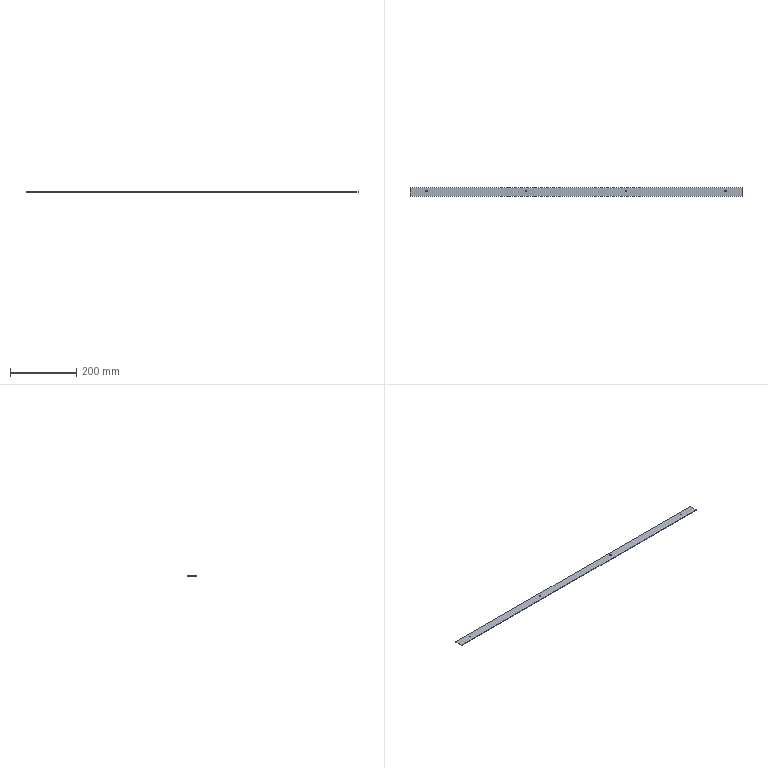Part | STEP file | 1 solid | 14 faces | box 1000 x 25 x 1.5 mm | volume 37405 mm3 | cylinder 8 | plane 6 | commonest cylinder face diameters 4.5 x8
STEP:
#1=CARTESIAN_POINT('',(0.,0.,0.));
#2=DIRECTION('',(0.,0.,1.));
#3=DIRECTION('',(1.,0.,0.));
#4=AXIS2_PLACEMENT_3D('',#1,#2,#3);
#5=CARTESIAN_POINT('',(782.25,-55.,1.5));
#6=VERTEX_POINT('',#5);
#7=CARTESIAN_POINT('',(777.75,-55.,1.5));
#8=VERTEX_POINT('',#7);
#9=CARTESIAN_POINT('',(780.,-55.,1.5));
#10=DIRECTION('',(0.,0.,1.));
#11=DIRECTION('',(1.,0.,0.));
#12=AXIS2_PLACEMENT_3D('',#9,#10,#11);
#13=CIRCLE('',#12,2.25);
#14=CARTESIAN_POINT('',(780.,-55.,1.5));
#15=DIRECTION('',(0.,0.,1.));
#16=DIRECTION('',(1.,0.,0.));
#17=AXIS2_PLACEMENT_3D('',#14,#15,#16);
#18=CYLINDRICAL_SURFACE('',#17,2.25);
#19=CARTESIAN_POINT('',(0.,0.));
#20=DIRECTION('',(1.,0.));
#21=VECTOR('',#20,1.);
#22=LINE('',#19,#21);
#23=(GEOMETRIC_REPRESENTATION_CONTEXT(2)PARAMETRIC_REPRESENTATION_CONTEXT()REPRESENTATION_CONTEXT('',''));
#24=DEFINITIONAL_REPRESENTATION('',(#22),#23);
#25=PCURVE('',#18,#24);
#26=CARTESIAN_POINT('',(0.,0.,1.5));
#27=DIRECTION('',(0.,0.,1.));
#28=DIRECTION('',(1.,0.,0.));
#29=AXIS2_PLACEMENT_3D('',#26,#27,#28);
#30=PLANE('',#29);
#31=CARTESIAN_POINT('',(780.,-55.));
#32=DIRECTION('',(1.,0.));
#33=AXIS2_PLACEMENT_2D('',#31,#32);
#34=CIRCLE('',#33,2.25);
#35=(GEOMETRIC_REPRESENTATION_CONTEXT(2)PARAMETRIC_REPRESENTATION_CONTEXT()REPRESENTATION_CONTEXT('',''));
#36=DEFINITIONAL_REPRESENTATION('',(#34),#35);
#37=PCURVE('',#30,#36);
#38=SURFACE_CURVE('',#13,(#25,#37),.PCURVE_S1.);
#39=EDGE_CURVE('',#6,#8,#38,.T.);
#40=ORIENTED_EDGE('',*,*,#39,.F.);
#41=CARTESIAN_POINT('',(782.25,-55.,0.));
#42=VERTEX_POINT('',#41);
#43=CARTESIAN_POINT('',(782.25,-55.,1.5));
#44=DIRECTION('',(0.,0.,1.));
#45=VECTOR('',#44,1.);
#46=LINE('',#43,#45);
#47=CARTESIAN_POINT('',(0.,0.));
#48=DIRECTION('',(0.,1.));
#49=VECTOR('',#48,1.);
#50=LINE('',#47,#49);
#51=(GEOMETRIC_REPRESENTATION_CONTEXT(2)PARAMETRIC_REPRESENTATION_CONTEXT()REPRESENTATION_CONTEXT('',''));
#52=DEFINITIONAL_REPRESENTATION('',(#50),#51);
#53=PCURVE('',#18,#52);
#54=CARTESIAN_POINT('',(780.,-55.,1.5));
#55=DIRECTION('',(0.,0.,1.));
#56=DIRECTION('',(1.,0.,0.));
#57=AXIS2_PLACEMENT_3D('',#54,#55,#56);
#58=CYLINDRICAL_SURFACE('',#57,2.25);
#59=CARTESIAN_POINT('',(6.283,0.));
#60=DIRECTION('',(0.,1.));
#61=VECTOR('',#60,1.);
#62=LINE('',#59,#61);
#63=(GEOMETRIC_REPRESENTATION_CONTEXT(2)PARAMETRIC_REPRESENTATION_CONTEXT()REPRESENTATION_CONTEXT('',''));
#64=DEFINITIONAL_REPRESENTATION('',(#62),#63);
#65=PCURVE('',#58,#64);
#66=SURFACE_CURVE('',#46,(#53,#65),.PCURVE_S1.);
#67=EDGE_CURVE('',#42,#6,#66,.T.);
#68=ORIENTED_EDGE('',*,*,#67,.F.);
#69=CARTESIAN_POINT('',(777.75,-55.,0.));
#70=VERTEX_POINT('',#69);
#71=CARTESIAN_POINT('',(780.,-55.,0.));
#72=DIRECTION('',(0.,0.,1.));
#73=DIRECTION('',(1.,0.,0.));
#74=AXIS2_PLACEMENT_3D('',#71,#72,#73);
#75=CIRCLE('',#74,2.25);
#76=CARTESIAN_POINT('',(0.,-1.5));
#77=DIRECTION('',(1.,0.));
#78=VECTOR('',#77,1.);
#79=LINE('',#76,#78);
#80=(GEOMETRIC_REPRESENTATION_CONTEXT(2)PARAMETRIC_REPRESENTATION_CONTEXT()REPRESENTATION_CONTEXT('',''));
#81=DEFINITIONAL_REPRESENTATION('',(#79),#80);
#82=PCURVE('',#18,#81);
#83=CARTESIAN_POINT('',(0.,0.,0.));
#84=DIRECTION('',(0.,0.,1.));
#85=DIRECTION('',(1.,0.,0.));
#86=AXIS2_PLACEMENT_3D('',#83,#84,#85);
#87=PLANE('',#86);
#88=CARTESIAN_POINT('',(780.,-55.));
#89=DIRECTION('',(1.,0.));
#90=AXIS2_PLACEMENT_2D('',#88,#89);
#91=CIRCLE('',#90,2.25);
#92=(GEOMETRIC_REPRESENTATION_CONTEXT(2)PARAMETRIC_REPRESENTATION_CONTEXT()REPRESENTATION_CONTEXT('',''));
#93=DEFINITIONAL_REPRESENTATION('',(#91),#92);
#94=PCURVE('',#87,#93);
#95=SURFACE_CURVE('',#75,(#82,#94),.PCURVE_S1.);
#96=EDGE_CURVE('',#42,#70,#95,.T.);
#97=ORIENTED_EDGE('',*,*,#96,.T.);
#98=CARTESIAN_POINT('',(777.75,-55.,1.5));
#99=DIRECTION('',(0.,0.,1.));
#100=VECTOR('',#99,1.);
#101=LINE('',#98,#100);
#102=CARTESIAN_POINT('',(3.142,0.));
#103=DIRECTION('',(0.,1.));
#104=VECTOR('',#103,1.);
#105=LINE('',#102,#104);
#106=(GEOMETRIC_REPRESENTATION_CONTEXT(2)PARAMETRIC_REPRESENTATION_CONTEXT()REPRESENTATION_CONTEXT('',''));
#107=DEFINITIONAL_REPRESENTATION('',(#105),#106);
#108=PCURVE('',#18,#107);
#109=CARTESIAN_POINT('',(3.142,0.));
#110=DIRECTION('',(0.,1.));
#111=VECTOR('',#110,1.);
#112=LINE('',#109,#111);
#113=(GEOMETRIC_REPRESENTATION_CONTEXT(2)PARAMETRIC_REPRESENTATION_CONTEXT()REPRESENTATION_CONTEXT('',''));
#114=DEFINITIONAL_REPRESENTATION('',(#112),#113);
#115=PCURVE('',#58,#114);
#116=SURFACE_CURVE('',#101,(#108,#115),.PCURVE_S1.);
#117=EDGE_CURVE('',#70,#8,#116,.T.);
#118=ORIENTED_EDGE('',*,*,#117,.T.);
#119=EDGE_LOOP('',(#40,#68,#97,#118));
#120=FACE_BOUND('',#119,.F.);
#121=ADVANCED_FACE('',(#120),#18,.F.);
#122=CARTESIAN_POINT('',(1082.25,-55.,1.5));
#123=VERTEX_POINT('',#122);
#124=CARTESIAN_POINT('',(1077.75,-55.,1.5));
#125=VERTEX_POINT('',#124);
#126=CARTESIAN_POINT('',(1080.,-55.,1.5));
#127=DIRECTION('',(0.,0.,1.));
#128=DIRECTION('',(1.,0.,0.));
#129=AXIS2_PLACEMENT_3D('',#126,#127,#128);
#130=CIRCLE('',#129,2.25);
#131=CARTESIAN_POINT('',(1080.,-55.,1.5));
#132=DIRECTION('',(0.,0.,1.));
#133=DIRECTION('',(1.,0.,0.));
#134=AXIS2_PLACEMENT_3D('',#131,#132,#133);
#135=CYLINDRICAL_SURFACE('',#134,2.25);
#136=CARTESIAN_POINT('',(0.,0.));
#137=DIRECTION('',(1.,0.));
#138=VECTOR('',#137,1.);
#139=LINE('',#136,#138);
#140=(GEOMETRIC_REPRESENTATION_CONTEXT(2)PARAMETRIC_REPRESENTATION_CONTEXT()REPRESENTATION_CONTEXT('',''));
#141=DEFINITIONAL_REPRESENTATION('',(#139),#140);
#142=PCURVE('',#135,#141);
#143=CARTESIAN_POINT('',(1080.,-55.));
#144=DIRECTION('',(1.,0.));
#145=AXIS2_PLACEMENT_2D('',#143,#144);
#146=CIRCLE('',#145,2.25);
#147=(GEOMETRIC_REPRESENTATION_CONTEXT(2)PARAMETRIC_REPRESENTATION_CONTEXT()REPRESENTATION_CONTEXT('',''));
#148=DEFINITIONAL_REPRESENTATION('',(#146),#147);
#149=PCURVE('',#30,#148);
#150=SURFACE_CURVE('',#130,(#142,#149),.PCURVE_S1.);
#151=EDGE_CURVE('',#123,#125,#150,.T.);
#152=ORIENTED_EDGE('',*,*,#151,.F.);
#153=CARTESIAN_POINT('',(1082.25,-55.,0.));
#154=VERTEX_POINT('',#153);
#155=CARTESIAN_POINT('',(1082.25,-55.,1.5));
#156=DIRECTION('',(0.,0.,1.));
#157=VECTOR('',#156,1.);
#158=LINE('',#155,#157);
#159=CARTESIAN_POINT('',(0.,0.));
#160=DIRECTION('',(0.,1.));
#161=VECTOR('',#160,1.);
#162=LINE('',#159,#161);
#163=(GEOMETRIC_REPRESENTATION_CONTEXT(2)PARAMETRIC_REPRESENTATION_CONTEXT()REPRESENTATION_CONTEXT('',''));
#164=DEFINITIONAL_REPRESENTATION('',(#162),#163);
#165=PCURVE('',#135,#164);
#166=CARTESIAN_POINT('',(1080.,-55.,1.5));
#167=DIRECTION('',(0.,0.,1.));
#168=DIRECTION('',(1.,0.,0.));
#169=AXIS2_PLACEMENT_3D('',#166,#167,#168);
#170=CYLINDRICAL_SURFACE('',#169,2.25);
#171=CARTESIAN_POINT('',(6.283,0.));
#172=DIRECTION('',(0.,1.));
#173=VECTOR('',#172,1.);
#174=LINE('',#171,#173);
#175=(GEOMETRIC_REPRESENTATION_CONTEXT(2)PARAMETRIC_REPRESENTATION_CONTEXT()REPRESENTATION_CONTEXT('',''));
#176=DEFINITIONAL_REPRESENTATION('',(#174),#175);
#177=PCURVE('',#170,#176);
#178=SURFACE_CURVE('',#158,(#165,#177),.PCURVE_S1.);
#179=EDGE_CURVE('',#154,#123,#178,.T.);
#180=ORIENTED_EDGE('',*,*,#179,.F.);
#181=CARTESIAN_POINT('',(1077.75,-55.,0.));
#182=VERTEX_POINT('',#181);
#183=CARTESIAN_POINT('',(1080.,-55.,0.));
#184=DIRECTION('',(0.,0.,1.));
#185=DIRECTION('',(1.,0.,0.));
#186=AXIS2_PLACEMENT_3D('',#183,#184,#185);
#187=CIRCLE('',#186,2.25);
#188=CARTESIAN_POINT('',(0.,-1.5));
#189=DIRECTION('',(1.,0.));
#190=VECTOR('',#189,1.);
#191=LINE('',#188,#190);
#192=(GEOMETRIC_REPRESENTATION_CONTEXT(2)PARAMETRIC_REPRESENTATION_CONTEXT()REPRESENTATION_CONTEXT('',''));
#193=DEFINITIONAL_REPRESENTATION('',(#191),#192);
#194=PCURVE('',#135,#193);
#195=CARTESIAN_POINT('',(1080.,-55.));
#196=DIRECTION('',(1.,0.));
#197=AXIS2_PLACEMENT_2D('',#195,#196);
#198=CIRCLE('',#197,2.25);
#199=(GEOMETRIC_REPRESENTATION_CONTEXT(2)PARAMETRIC_REPRESENTATION_CONTEXT()REPRESENTATION_CONTEXT('',''));
#200=DEFINITIONAL_REPRESENTATION('',(#198),#199);
#201=PCURVE('',#87,#200);
#202=SURFACE_CURVE('',#187,(#194,#201),.PCURVE_S1.);
#203=EDGE_CURVE('',#154,#182,#202,.T.);
#204=ORIENTED_EDGE('',*,*,#203,.T.);
#205=CARTESIAN_POINT('',(1077.75,-55.,1.5));
#206=DIRECTION('',(0.,0.,1.));
#207=VECTOR('',#206,1.);
#208=LINE('',#205,#207);
#209=CARTESIAN_POINT('',(3.142,0.));
#210=DIRECTION('',(0.,1.));
#211=VECTOR('',#210,1.);
#212=LINE('',#209,#211);
#213=(GEOMETRIC_REPRESENTATION_CONTEXT(2)PARAMETRIC_REPRESENTATION_CONTEXT()REPRESENTATION_CONTEXT('',''));
#214=DEFINITIONAL_REPRESENTATION('',(#212),#213);
#215=PCURVE('',#135,#214);
#216=CARTESIAN_POINT('',(3.142,0.));
#217=DIRECTION('',(0.,1.));
#218=VECTOR('',#217,1.);
#219=LINE('',#216,#218);
#220=(GEOMETRIC_REPRESENTATION_CONTEXT(2)PARAMETRIC_REPRESENTATION_CONTEXT()REPRESENTATION_CONTEXT('',''));
#221=DEFINITIONAL_REPRESENTATION('',(#219),#220);
#222=PCURVE('',#170,#221);
#223=SURFACE_CURVE('',#208,(#215,#222),.PCURVE_S1.);
#224=EDGE_CURVE('',#182,#125,#223,.T.);
#225=ORIENTED_EDGE('',*,*,#224,.T.);
#226=EDGE_LOOP('',(#152,#180,#204,#225));
#227=FACE_BOUND('',#226,.F.);
#228=ADVANCED_FACE('',(#227),#135,.F.);
#229=CARTESIAN_POINT('',(1382.25,-55.,1.5));
#230=VERTEX_POINT('',#229);
#231=CARTESIAN_POINT('',(1377.75,-55.,1.5));
#232=VERTEX_POINT('',#231);
#233=CARTESIAN_POINT('',(1380.,-55.,1.5));
#234=DIRECTION('',(0.,0.,1.));
#235=DIRECTION('',(1.,0.,0.));
#236=AXIS2_PLACEMENT_3D('',#233,#234,#235);
#237=CIRCLE('',#236,2.25);
#238=CARTESIAN_POINT('',(1380.,-55.,1.5));
#239=DIRECTION('',(0.,0.,1.));
#240=DIRECTION('',(1.,0.,0.));
#241=AXIS2_PLACEMENT_3D('',#238,#239,#240);
#242=CYLINDRICAL_SURFACE('',#241,2.25);
#243=CARTESIAN_POINT('',(0.,0.));
#244=DIRECTION('',(1.,0.));
#245=VECTOR('',#244,1.);
#246=LINE('',#243,#245);
#247=(GEOMETRIC_REPRESENTATION_CONTEXT(2)PARAMETRIC_REPRESENTATION_CONTEXT()REPRESENTATION_CONTEXT('',''));
#248=DEFINITIONAL_REPRESENTATION('',(#246),#247);
#249=PCURVE('',#242,#248);
#250=CARTESIAN_POINT('',(1380.,-55.));
#251=DIRECTION('',(1.,0.));
#252=AXIS2_PLACEMENT_2D('',#250,#251);
#253=CIRCLE('',#252,2.25);
#254=(GEOMETRIC_REPRESENTATION_CONTEXT(2)PARAMETRIC_REPRESENTATION_CONTEXT()REPRESENTATION_CONTEXT('',''));
#255=DEFINITIONAL_REPRESENTATION('',(#253),#254);
#256=PCURVE('',#30,#255);
#257=SURFACE_CURVE('',#237,(#249,#256),.PCURVE_S1.);
#258=EDGE_CURVE('',#230,#232,#257,.T.);
#259=ORIENTED_EDGE('',*,*,#258,.F.);
#260=CARTESIAN_POINT('',(1382.25,-55.,0.));
#261=VERTEX_POINT('',#260);
#262=CARTESIAN_POINT('',(1382.25,-55.,1.5));
#263=DIRECTION('',(0.,0.,1.));
#264=VECTOR('',#263,1.);
#265=LINE('',#262,#264);
#266=CARTESIAN_POINT('',(0.,0.));
#267=DIRECTION('',(0.,1.));
#268=VECTOR('',#267,1.);
#269=LINE('',#266,#268);
#270=(GEOMETRIC_REPRESENTATION_CONTEXT(2)PARAMETRIC_REPRESENTATION_CONTEXT()REPRESENTATION_CONTEXT('',''));
#271=DEFINITIONAL_REPRESENTATION('',(#269),#270);
#272=PCURVE('',#242,#271);
#273=CARTESIAN_POINT('',(1380.,-55.,1.5));
#274=DIRECTION('',(0.,0.,1.));
#275=DIRECTION('',(1.,0.,0.));
#276=AXIS2_PLACEMENT_3D('',#273,#274,#275);
#277=CYLINDRICAL_SURFACE('',#276,2.25);
#278=CARTESIAN_POINT('',(6.283,0.));
#279=DIRECTION('',(0.,1.));
#280=VECTOR('',#279,1.);
#281=LINE('',#278,#280);
#282=(GEOMETRIC_REPRESENTATION_CONTEXT(2)PARAMETRIC_REPRESENTATION_CONTEXT()REPRESENTATION_CONTEXT('',''));
#283=DEFINITIONAL_REPRESENTATION('',(#281),#282);
#284=PCURVE('',#277,#283);
#285=SURFACE_CURVE('',#265,(#272,#284),.PCURVE_S1.);
#286=EDGE_CURVE('',#261,#230,#285,.T.);
#287=ORIENTED_EDGE('',*,*,#286,.F.);
#288=CARTESIAN_POINT('',(1377.75,-55.,0.));
#289=VERTEX_POINT('',#288);
#290=CARTESIAN_POINT('',(1380.,-55.,0.));
#291=DIRECTION('',(0.,0.,1.));
#292=DIRECTION('',(1.,0.,0.));
#293=AXIS2_PLACEMENT_3D('',#290,#291,#292);
#294=CIRCLE('',#293,2.25);
#295=CARTESIAN_POINT('',(0.,-1.5));
#296=DIRECTION('',(1.,0.));
#297=VECTOR('',#296,1.);
#298=LINE('',#295,#297);
#299=(GEOMETRIC_REPRESENTATION_CONTEXT(2)PARAMETRIC_REPRESENTATION_CONTEXT()REPRESENTATION_CONTEXT('',''));
#300=DEFINITIONAL_REPRESENTATION('',(#298),#299);
#301=PCURVE('',#242,#300);
#302=CARTESIAN_POINT('',(1380.,-55.));
#303=DIRECTION('',(1.,0.));
#304=AXIS2_PLACEMENT_2D('',#302,#303);
#305=CIRCLE('',#304,2.25);
#306=(GEOMETRIC_REPRESENTATION_CONTEXT(2)PARAMETRIC_REPRESENTATION_CONTEXT()REPRESENTATION_CONTEXT('',''));
#307=DEFINITIONAL_REPRESENTATION('',(#305),#306);
#308=PCURVE('',#87,#307);
#309=SURFACE_CURVE('',#294,(#301,#308),.PCURVE_S1.);
#310=EDGE_CURVE('',#261,#289,#309,.T.);
#311=ORIENTED_EDGE('',*,*,#310,.T.);
#312=CARTESIAN_POINT('',(1377.75,-55.,1.5));
#313=DIRECTION('',(0.,0.,1.));
#314=VECTOR('',#313,1.);
#315=LINE('',#312,#314);
#316=CARTESIAN_POINT('',(3.142,0.));
#317=DIRECTION('',(0.,1.));
#318=VECTOR('',#317,1.);
#319=LINE('',#316,#318);
#320=(GEOMETRIC_REPRESENTATION_CONTEXT(2)PARAMETRIC_REPRESENTATION_CONTEXT()REPRESENTATION_CONTEXT('',''));
#321=DEFINITIONAL_REPRESENTATION('',(#319),#320);
#322=PCURVE('',#242,#321);
#323=CARTESIAN_POINT('',(3.142,0.));
#324=DIRECTION('',(0.,1.));
#325=VECTOR('',#324,1.);
#326=LINE('',#323,#325);
#327=(GEOMETRIC_REPRESENTATION_CONTEXT(2)PARAMETRIC_REPRESENTATION_CONTEXT()REPRESENTATION_CONTEXT('',''));
#328=DEFINITIONAL_REPRESENTATION('',(#326),#327);
#329=PCURVE('',#277,#328);
#330=SURFACE_CURVE('',#315,(#322,#329),.PCURVE_S1.);
#331=EDGE_CURVE('',#289,#232,#330,.T.);
#332=ORIENTED_EDGE('',*,*,#331,.T.);
#333=EDGE_LOOP('',(#259,#287,#311,#332));
#334=FACE_BOUND('',#333,.F.);
#335=ADVANCED_FACE('',(#334),#242,.F.);
#336=CARTESIAN_POINT('',(1682.25,-55.,1.5));
#337=VERTEX_POINT('',#336);
#338=CARTESIAN_POINT('',(1677.75,-55.,1.5));
#339=VERTEX_POINT('',#338);
#340=CARTESIAN_POINT('',(1680.,-55.,1.5));
#341=DIRECTION('',(0.,0.,1.));
#342=DIRECTION('',(1.,0.,0.));
#343=AXIS2_PLACEMENT_3D('',#340,#341,#342);
#344=CIRCLE('',#343,2.25);
#345=CARTESIAN_POINT('',(1680.,-55.,1.5));
#346=DIRECTION('',(0.,0.,1.));
#347=DIRECTION('',(1.,0.,0.));
#348=AXIS2_PLACEMENT_3D('',#345,#346,#347);
#349=CYLINDRICAL_SURFACE('',#348,2.25);
#350=CARTESIAN_POINT('',(0.,0.));
#351=DIRECTION('',(1.,0.));
#352=VECTOR('',#351,1.);
#353=LINE('',#350,#352);
#354=(GEOMETRIC_REPRESENTATION_CONTEXT(2)PARAMETRIC_REPRESENTATION_CONTEXT()REPRESENTATION_CONTEXT('',''));
#355=DEFINITIONAL_REPRESENTATION('',(#353),#354);
#356=PCURVE('',#349,#355);
#357=CARTESIAN_POINT('',(1680.,-55.));
#358=DIRECTION('',(1.,0.));
#359=AXIS2_PLACEMENT_2D('',#357,#358);
#360=CIRCLE('',#359,2.25);
#361=(GEOMETRIC_REPRESENTATION_CONTEXT(2)PARAMETRIC_REPRESENTATION_CONTEXT()REPRESENTATION_CONTEXT('',''));
#362=DEFINITIONAL_REPRESENTATION('',(#360),#361);
#363=PCURVE('',#30,#362);
#364=SURFACE_CURVE('',#344,(#356,#363),.PCURVE_S1.);
#365=EDGE_CURVE('',#337,#339,#364,.T.);
#366=ORIENTED_EDGE('',*,*,#365,.F.);
#367=CARTESIAN_POINT('',(1682.25,-55.,0.));
#368=VERTEX_POINT('',#367);
#369=CARTESIAN_POINT('',(1682.25,-55.,1.5));
#370=DIRECTION('',(0.,0.,1.));
#371=VECTOR('',#370,1.);
#372=LINE('',#369,#371);
#373=CARTESIAN_POINT('',(0.,0.));
#374=DIRECTION('',(0.,1.));
#375=VECTOR('',#374,1.);
#376=LINE('',#373,#375);
#377=(GEOMETRIC_REPRESENTATION_CONTEXT(2)PARAMETRIC_REPRESENTATION_CONTEXT()REPRESENTATION_CONTEXT('',''));
#378=DEFINITIONAL_REPRESENTATION('',(#376),#377);
#379=PCURVE('',#349,#378);
#380=CARTESIAN_POINT('',(1680.,-55.,1.5));
#381=DIRECTION('',(0.,0.,1.));
#382=DIRECTION('',(1.,0.,0.));
#383=AXIS2_PLACEMENT_3D('',#380,#381,#382);
#384=CYLINDRICAL_SURFACE('',#383,2.25);
#385=CARTESIAN_POINT('',(6.283,0.));
#386=DIRECTION('',(0.,1.));
#387=VECTOR('',#386,1.);
#388=LINE('',#385,#387);
#389=(GEOMETRIC_REPRESENTATION_CONTEXT(2)PARAMETRIC_REPRESENTATION_CONTEXT()REPRESENTATION_CONTEXT('',''));
#390=DEFINITIONAL_REPRESENTATION('',(#388),#389);
#391=PCURVE('',#384,#390);
#392=SURFACE_CURVE('',#372,(#379,#391),.PCURVE_S1.);
#393=EDGE_CURVE('',#368,#337,#392,.T.);
#394=ORIENTED_EDGE('',*,*,#393,.F.);
#395=CARTESIAN_POINT('',(1677.75,-55.,0.));
#396=VERTEX_POINT('',#395);
#397=CARTESIAN_POINT('',(1680.,-55.,0.));
#398=DIRECTION('',(0.,0.,1.));
#399=DIRECTION('',(1.,0.,0.));
#400=AXIS2_PLACEMENT_3D('',#397,#398,#399);
#401=CIRCLE('',#400,2.25);
#402=CARTESIAN_POINT('',(0.,-1.5));
#403=DIRECTION('',(1.,0.));
#404=VECTOR('',#403,1.);
#405=LINE('',#402,#404);
#406=(GEOMETRIC_REPRESENTATION_CONTEXT(2)PARAMETRIC_REPRESENTATION_CONTEXT()REPRESENTATION_CONTEXT('',''));
#407=DEFINITIONAL_REPRESENTATION('',(#405),#406);
#408=PCURVE('',#349,#407);
#409=CARTESIAN_POINT('',(1680.,-55.));
#410=DIRECTION('',(1.,0.));
#411=AXIS2_PLACEMENT_2D('',#409,#410);
#412=CIRCLE('',#411,2.25);
#413=(GEOMETRIC_REPRESENTATION_CONTEXT(2)PARAMETRIC_REPRESENTATION_CONTEXT()REPRESENTATION_CONTEXT('',''));
#414=DEFINITIONAL_REPRESENTATION('',(#412),#413);
#415=PCURVE('',#87,#414);
#416=SURFACE_CURVE('',#401,(#408,#415),.PCURVE_S1.);
#417=EDGE_CURVE('',#368,#396,#416,.T.);
#418=ORIENTED_EDGE('',*,*,#417,.T.);
#419=CARTESIAN_POINT('',(1677.75,-55.,1.5));
#420=DIRECTION('',(0.,0.,1.));
#421=VECTOR('',#420,1.);
#422=LINE('',#419,#421);
#423=CARTESIAN_POINT('',(3.142,0.));
#424=DIRECTION('',(0.,1.));
#425=VECTOR('',#424,1.);
#426=LINE('',#423,#425);
#427=(GEOMETRIC_REPRESENTATION_CONTEXT(2)PARAMETRIC_REPRESENTATION_CONTEXT()REPRESENTATION_CONTEXT('',''));
#428=DEFINITIONAL_REPRESENTATION('',(#426),#427);
#429=PCURVE('',#349,#428);
#430=CARTESIAN_POINT('',(3.142,0.));
#431=DIRECTION('',(0.,1.));
#432=VECTOR('',#431,1.);
#433=LINE('',#430,#432);
#434=(GEOMETRIC_REPRESENTATION_CONTEXT(2)PARAMETRIC_REPRESENTATION_CONTEXT()REPRESENTATION_CONTEXT('',''));
#435=DEFINITIONAL_REPRESENTATION('',(#433),#434);
#436=PCURVE('',#384,#435);
#437=SURFACE_CURVE('',#422,(#429,#436),.PCURVE_S1.);
#438=EDGE_CURVE('',#396,#339,#437,.T.);
#439=ORIENTED_EDGE('',*,*,#438,.T.);
#440=EDGE_LOOP('',(#366,#394,#418,#439));
#441=FACE_BOUND('',#440,.F.);
#442=ADVANCED_FACE('',(#441),#349,.F.);
#443=ORIENTED_EDGE('',*,*,#417,.T.);
#444=CARTESIAN_POINT('',(1680.,-55.,0.));
#445=DIRECTION('',(0.,0.,1.));
#446=DIRECTION('',(1.,0.,0.));
#447=AXIS2_PLACEMENT_3D('',#444,#445,#446);
#448=CIRCLE('',#447,2.25);
#449=CARTESIAN_POINT('',(1680.,-55.));
#450=DIRECTION('',(1.,0.));
#451=AXIS2_PLACEMENT_2D('',#449,#450);
#452=CIRCLE('',#451,2.25);
#453=(GEOMETRIC_REPRESENTATION_CONTEXT(2)PARAMETRIC_REPRESENTATION_CONTEXT()REPRESENTATION_CONTEXT('',''));
#454=DEFINITIONAL_REPRESENTATION('',(#452),#453);
#455=PCURVE('',#87,#454);
#456=CARTESIAN_POINT('',(0.,-1.5));
#457=DIRECTION('',(1.,0.));
#458=VECTOR('',#457,1.);
#459=LINE('',#456,#458);
#460=(GEOMETRIC_REPRESENTATION_CONTEXT(2)PARAMETRIC_REPRESENTATION_CONTEXT()REPRESENTATION_CONTEXT('',''));
#461=DEFINITIONAL_REPRESENTATION('',(#459),#460);
#462=PCURVE('',#384,#461);
#463=SURFACE_CURVE('',#448,(#455,#462),.PCURVE_S1.);
#464=EDGE_CURVE('',#396,#368,#463,.T.);
#465=ORIENTED_EDGE('',*,*,#464,.T.);
#466=EDGE_LOOP('',(#443,#465));
#467=FACE_BOUND('',#466,.T.);
#468=ORIENTED_EDGE('',*,*,#310,.T.);
#469=CARTESIAN_POINT('',(1380.,-55.,0.));
#470=DIRECTION('',(0.,0.,1.));
#471=DIRECTION('',(1.,0.,0.));
#472=AXIS2_PLACEMENT_3D('',#469,#470,#471);
#473=CIRCLE('',#472,2.25);
#474=CARTESIAN_POINT('',(1380.,-55.));
#475=DIRECTION('',(1.,0.));
#476=AXIS2_PLACEMENT_2D('',#474,#475);
#477=CIRCLE('',#476,2.25);
#478=(GEOMETRIC_REPRESENTATION_CONTEXT(2)PARAMETRIC_REPRESENTATION_CONTEXT()REPRESENTATION_CONTEXT('',''));
#479=DEFINITIONAL_REPRESENTATION('',(#477),#478);
#480=PCURVE('',#87,#479);
#481=CARTESIAN_POINT('',(0.,-1.5));
#482=DIRECTION('',(1.,0.));
#483=VECTOR('',#482,1.);
#484=LINE('',#481,#483);
#485=(GEOMETRIC_REPRESENTATION_CONTEXT(2)PARAMETRIC_REPRESENTATION_CONTEXT()REPRESENTATION_CONTEXT('',''));
#486=DEFINITIONAL_REPRESENTATION('',(#484),#485);
#487=PCURVE('',#277,#486);
#488=SURFACE_CURVE('',#473,(#480,#487),.PCURVE_S1.);
#489=EDGE_CURVE('',#289,#261,#488,.T.);
#490=ORIENTED_EDGE('',*,*,#489,.T.);
#491=EDGE_LOOP('',(#468,#490));
#492=FACE_BOUND('',#491,.T.);
#493=ORIENTED_EDGE('',*,*,#203,.T.);
#494=CARTESIAN_POINT('',(1080.,-55.,0.));
#495=DIRECTION('',(0.,0.,1.));
#496=DIRECTION('',(1.,0.,0.));
#497=AXIS2_PLACEMENT_3D('',#494,#495,#496);
#498=CIRCLE('',#497,2.25);
#499=CARTESIAN_POINT('',(1080.,-55.));
#500=DIRECTION('',(1.,0.));
#501=AXIS2_PLACEMENT_2D('',#499,#500);
#502=CIRCLE('',#501,2.25);
#503=(GEOMETRIC_REPRESENTATION_CONTEXT(2)PARAMETRIC_REPRESENTATION_CONTEXT()REPRESENTATION_CONTEXT('',''));
#504=DEFINITIONAL_REPRESENTATION('',(#502),#503);
#505=PCURVE('',#87,#504);
#506=CARTESIAN_POINT('',(0.,-1.5));
#507=DIRECTION('',(1.,0.));
#508=VECTOR('',#507,1.);
#509=LINE('',#506,#508);
#510=(GEOMETRIC_REPRESENTATION_CONTEXT(2)PARAMETRIC_REPRESENTATION_CONTEXT()REPRESENTATION_CONTEXT('',''));
#511=DEFINITIONAL_REPRESENTATION('',(#509),#510);
#512=PCURVE('',#170,#511);
#513=SURFACE_CURVE('',#498,(#505,#512),.PCURVE_S1.);
#514=EDGE_CURVE('',#182,#154,#513,.T.);
#515=ORIENTED_EDGE('',*,*,#514,.T.);
#516=EDGE_LOOP('',(#493,#515));
#517=FACE_BOUND('',#516,.T.);
#518=ORIENTED_EDGE('',*,*,#96,.T.);
#519=CARTESIAN_POINT('',(780.,-55.,0.));
#520=DIRECTION('',(0.,0.,1.));
#521=DIRECTION('',(1.,0.,0.));
#522=AXIS2_PLACEMENT_3D('',#519,#520,#521);
#523=CIRCLE('',#522,2.25);
#524=CARTESIAN_POINT('',(780.,-55.));
#525=DIRECTION('',(1.,0.));
#526=AXIS2_PLACEMENT_2D('',#524,#525);
#527=CIRCLE('',#526,2.25);
#528=(GEOMETRIC_REPRESENTATION_CONTEXT(2)PARAMETRIC_REPRESENTATION_CONTEXT()REPRESENTATION_CONTEXT('',''));
#529=DEFINITIONAL_REPRESENTATION('',(#527),#528);
#530=PCURVE('',#87,#529);
#531=CARTESIAN_POINT('',(0.,-1.5));
#532=DIRECTION('',(1.,0.));
#533=VECTOR('',#532,1.);
#534=LINE('',#531,#533);
#535=(GEOMETRIC_REPRESENTATION_CONTEXT(2)PARAMETRIC_REPRESENTATION_CONTEXT()REPRESENTATION_CONTEXT('',''));
#536=DEFINITIONAL_REPRESENTATION('',(#534),#535);
#537=PCURVE('',#58,#536);
#538=SURFACE_CURVE('',#523,(#530,#537),.PCURVE_S1.);
#539=EDGE_CURVE('',#70,#42,#538,.T.);
#540=ORIENTED_EDGE('',*,*,#539,.T.);
#541=EDGE_LOOP('',(#518,#540));
#542=FACE_BOUND('',#541,.T.);
#543=CARTESIAN_POINT('',(1730.,-45.,0.));
#544=VERTEX_POINT('',#543);
#545=CARTESIAN_POINT('',(730.,-45.,0.));
#546=VERTEX_POINT('',#545);
#547=CARTESIAN_POINT('',(1500.,-45.,0.));
#548=DIRECTION('',(-1.,0.,0.));
#549=VECTOR('',#548,1.);
#550=LINE('',#547,#549);
#551=CARTESIAN_POINT('',(1500.,-45.));
#552=DIRECTION('',(-1.,0.));
#553=VECTOR('',#552,1.);
#554=LINE('',#551,#553);
#555=(GEOMETRIC_REPRESENTATION_CONTEXT(2)PARAMETRIC_REPRESENTATION_CONTEXT()REPRESENTATION_CONTEXT('',''));
#556=DEFINITIONAL_REPRESENTATION('',(#554),#555);
#557=PCURVE('',#87,#556);
#558=CARTESIAN_POINT('',(1500.,-45.,1.5));
#559=DIRECTION('',(0.,-1.,0.));
#560=DIRECTION('',(0.,0.,-1.));
#561=AXIS2_PLACEMENT_3D('',#558,#559,#560);
#562=PLANE('',#561);
#563=CARTESIAN_POINT('',(1.5,0.));
#564=DIRECTION('',(0.,-1.));
#565=VECTOR('',#564,1.);
#566=LINE('',#563,#565);
#567=(GEOMETRIC_REPRESENTATION_CONTEXT(2)PARAMETRIC_REPRESENTATION_CONTEXT()REPRESENTATION_CONTEXT('',''));
#568=DEFINITIONAL_REPRESENTATION('',(#566),#567);
#569=PCURVE('',#562,#568);
#570=SURFACE_CURVE('',#550,(#557,#569),.PCURVE_S1.);
#571=EDGE_CURVE('',#544,#546,#570,.T.);
#572=ORIENTED_EDGE('',*,*,#571,.F.);
#573=CARTESIAN_POINT('',(1730.,-70.,0.));
#574=VERTEX_POINT('',#573);
#575=CARTESIAN_POINT('',(1730.,-70.,0.));
#576=DIRECTION('',(0.,1.,0.));
#577=VECTOR('',#576,1.);
#578=LINE('',#575,#577);
#579=CARTESIAN_POINT('',(1730.,-70.));
#580=DIRECTION('',(0.,1.));
#581=VECTOR('',#580,1.);
#582=LINE('',#579,#581);
#583=(GEOMETRIC_REPRESENTATION_CONTEXT(2)PARAMETRIC_REPRESENTATION_CONTEXT()REPRESENTATION_CONTEXT('',''));
#584=DEFINITIONAL_REPRESENTATION('',(#582),#583);
#585=PCURVE('',#87,#584);
#586=CARTESIAN_POINT('',(1730.,-70.,1.5));
#587=DIRECTION('',(-1.,0.,0.));
#588=DIRECTION('',(0.,0.,1.));
#589=AXIS2_PLACEMENT_3D('',#586,#587,#588);
#590=PLANE('',#589);
#591=CARTESIAN_POINT('',(-1.5,0.));
#592=DIRECTION('',(0.,1.));
#593=VECTOR('',#592,1.);
#594=LINE('',#591,#593);
#595=(GEOMETRIC_REPRESENTATION_CONTEXT(2)PARAMETRIC_REPRESENTATION_CONTEXT()REPRESENTATION_CONTEXT('',''));
#596=DEFINITIONAL_REPRESENTATION('',(#594),#595);
#597=PCURVE('',#590,#596);
#598=SURFACE_CURVE('',#578,(#585,#597),.PCURVE_S1.);
#599=EDGE_CURVE('',#574,#544,#598,.T.);
#600=ORIENTED_EDGE('',*,*,#599,.F.);
#601=CARTESIAN_POINT('',(730.,-70.,0.));
#602=VERTEX_POINT('',#601);
#603=CARTESIAN_POINT('',(600.,-70.,0.));
#604=DIRECTION('',(1.,0.,0.));
#605=VECTOR('',#604,1.);
#606=LINE('',#603,#605);
#607=CARTESIAN_POINT('',(600.,-70.));
#608=DIRECTION('',(1.,0.));
#609=VECTOR('',#608,1.);
#610=LINE('',#607,#609);
#611=(GEOMETRIC_REPRESENTATION_CONTEXT(2)PARAMETRIC_REPRESENTATION_CONTEXT()REPRESENTATION_CONTEXT('',''));
#612=DEFINITIONAL_REPRESENTATION('',(#610),#611);
#613=PCURVE('',#87,#612);
#614=CARTESIAN_POINT('',(600.,-70.,1.5));
#615=DIRECTION('',(0.,1.,0.));
#616=DIRECTION('',(1.,0.,0.));
#617=AXIS2_PLACEMENT_3D('',#614,#615,#616);
#618=PLANE('',#617);
#619=CARTESIAN_POINT('',(0.,1.5));
#620=DIRECTION('',(1.,0.));
#621=VECTOR('',#620,1.);
#622=LINE('',#619,#621);
#623=(GEOMETRIC_REPRESENTATION_CONTEXT(2)PARAMETRIC_REPRESENTATION_CONTEXT()REPRESENTATION_CONTEXT('',''));
#624=DEFINITIONAL_REPRESENTATION('',(#622),#623);
#625=PCURVE('',#618,#624);
#626=SURFACE_CURVE('',#606,(#613,#625),.PCURVE_S1.);
#627=EDGE_CURVE('',#602,#574,#626,.T.);
#628=ORIENTED_EDGE('',*,*,#627,.F.);
#629=CARTESIAN_POINT('',(730.,-45.,0.));
#630=DIRECTION('',(0.,-1.,0.));
#631=VECTOR('',#630,1.);
#632=LINE('',#629,#631);
#633=CARTESIAN_POINT('',(730.,-45.));
#634=DIRECTION('',(0.,-1.));
#635=VECTOR('',#634,1.);
#636=LINE('',#633,#635);
#637=(GEOMETRIC_REPRESENTATION_CONTEXT(2)PARAMETRIC_REPRESENTATION_CONTEXT()REPRESENTATION_CONTEXT('',''));
#638=DEFINITIONAL_REPRESENTATION('',(#636),#637);
#639=PCURVE('',#87,#638);
#640=CARTESIAN_POINT('',(730.,-45.,1.5));
#641=DIRECTION('',(1.,0.,0.));
#642=DIRECTION('',(0.,0.,1.));
#643=AXIS2_PLACEMENT_3D('',#640,#641,#642);
#644=PLANE('',#643);
#645=CARTESIAN_POINT('',(-1.5,0.));
#646=DIRECTION('',(0.,1.));
#647=VECTOR('',#646,1.);
#648=LINE('',#645,#647);
#649=(GEOMETRIC_REPRESENTATION_CONTEXT(2)PARAMETRIC_REPRESENTATION_CONTEXT()REPRESENTATION_CONTEXT('',''));
#650=DEFINITIONAL_REPRESENTATION('',(#648),#649);
#651=PCURVE('',#644,#650);
#652=SURFACE_CURVE('',#632,(#639,#651),.PCURVE_S1.);
#653=EDGE_CURVE('',#546,#602,#652,.T.);
#654=ORIENTED_EDGE('',*,*,#653,.F.);
#655=EDGE_LOOP('',(#572,#600,#628,#654));
#656=FACE_BOUND('',#655,.T.);
#657=ADVANCED_FACE('',(#467,#492,#517,#542,#656),#87,.F.);
#658=ORIENTED_EDGE('',*,*,#365,.F.);
#659=CARTESIAN_POINT('',(1680.,-55.,1.5));
#660=DIRECTION('',(0.,0.,1.));
#661=DIRECTION('',(1.,0.,0.));
#662=AXIS2_PLACEMENT_3D('',#659,#660,#661);
#663=CIRCLE('',#662,2.25);
#664=CARTESIAN_POINT('',(1680.,-55.));
#665=DIRECTION('',(1.,0.));
#666=AXIS2_PLACEMENT_2D('',#664,#665);
#667=CIRCLE('',#666,2.25);
#668=(GEOMETRIC_REPRESENTATION_CONTEXT(2)PARAMETRIC_REPRESENTATION_CONTEXT()REPRESENTATION_CONTEXT('',''));
#669=DEFINITIONAL_REPRESENTATION('',(#667),#668);
#670=PCURVE('',#30,#669);
#671=CARTESIAN_POINT('',(0.,0.));
#672=DIRECTION('',(1.,0.));
#673=VECTOR('',#672,1.);
#674=LINE('',#671,#673);
#675=(GEOMETRIC_REPRESENTATION_CONTEXT(2)PARAMETRIC_REPRESENTATION_CONTEXT()REPRESENTATION_CONTEXT('',''));
#676=DEFINITIONAL_REPRESENTATION('',(#674),#675);
#677=PCURVE('',#384,#676);
#678=SURFACE_CURVE('',#663,(#670,#677),.PCURVE_S1.);
#679=EDGE_CURVE('',#339,#337,#678,.T.);
#680=ORIENTED_EDGE('',*,*,#679,.F.);
#681=EDGE_LOOP('',(#658,#680));
#682=FACE_BOUND('',#681,.T.);
#683=ORIENTED_EDGE('',*,*,#258,.F.);
#684=CARTESIAN_POINT('',(1380.,-55.,1.5));
#685=DIRECTION('',(0.,0.,1.));
#686=DIRECTION('',(1.,0.,0.));
#687=AXIS2_PLACEMENT_3D('',#684,#685,#686);
#688=CIRCLE('',#687,2.25);
#689=CARTESIAN_POINT('',(1380.,-55.));
#690=DIRECTION('',(1.,0.));
#691=AXIS2_PLACEMENT_2D('',#689,#690);
#692=CIRCLE('',#691,2.25);
#693=(GEOMETRIC_REPRESENTATION_CONTEXT(2)PARAMETRIC_REPRESENTATION_CONTEXT()REPRESENTATION_CONTEXT('',''));
#694=DEFINITIONAL_REPRESENTATION('',(#692),#693);
#695=PCURVE('',#30,#694);
#696=CARTESIAN_POINT('',(0.,0.));
#697=DIRECTION('',(1.,0.));
#698=VECTOR('',#697,1.);
#699=LINE('',#696,#698);
#700=(GEOMETRIC_REPRESENTATION_CONTEXT(2)PARAMETRIC_REPRESENTATION_CONTEXT()REPRESENTATION_CONTEXT('',''));
#701=DEFINITIONAL_REPRESENTATION('',(#699),#700);
#702=PCURVE('',#277,#701);
#703=SURFACE_CURVE('',#688,(#695,#702),.PCURVE_S1.);
#704=EDGE_CURVE('',#232,#230,#703,.T.);
#705=ORIENTED_EDGE('',*,*,#704,.F.);
#706=EDGE_LOOP('',(#683,#705));
#707=FACE_BOUND('',#706,.T.);
#708=ORIENTED_EDGE('',*,*,#151,.F.);
#709=CARTESIAN_POINT('',(1080.,-55.,1.5));
#710=DIRECTION('',(0.,0.,1.));
#711=DIRECTION('',(1.,0.,0.));
#712=AXIS2_PLACEMENT_3D('',#709,#710,#711);
#713=CIRCLE('',#712,2.25);
#714=CARTESIAN_POINT('',(1080.,-55.));
#715=DIRECTION('',(1.,0.));
#716=AXIS2_PLACEMENT_2D('',#714,#715);
#717=CIRCLE('',#716,2.25);
#718=(GEOMETRIC_REPRESENTATION_CONTEXT(2)PARAMETRIC_REPRESENTATION_CONTEXT()REPRESENTATION_CONTEXT('',''));
#719=DEFINITIONAL_REPRESENTATION('',(#717),#718);
#720=PCURVE('',#30,#719);
#721=CARTESIAN_POINT('',(0.,0.));
#722=DIRECTION('',(1.,0.));
#723=VECTOR('',#722,1.);
#724=LINE('',#721,#723);
#725=(GEOMETRIC_REPRESENTATION_CONTEXT(2)PARAMETRIC_REPRESENTATION_CONTEXT()REPRESENTATION_CONTEXT('',''));
#726=DEFINITIONAL_REPRESENTATION('',(#724),#725);
#727=PCURVE('',#170,#726);
#728=SURFACE_CURVE('',#713,(#720,#727),.PCURVE_S1.);
#729=EDGE_CURVE('',#125,#123,#728,.T.);
#730=ORIENTED_EDGE('',*,*,#729,.F.);
#731=EDGE_LOOP('',(#708,#730));
#732=FACE_BOUND('',#731,.T.);
#733=ORIENTED_EDGE('',*,*,#39,.F.);
#734=CARTESIAN_POINT('',(780.,-55.,1.5));
#735=DIRECTION('',(0.,0.,1.));
#736=DIRECTION('',(1.,0.,0.));
#737=AXIS2_PLACEMENT_3D('',#734,#735,#736);
#738=CIRCLE('',#737,2.25);
#739=CARTESIAN_POINT('',(780.,-55.));
#740=DIRECTION('',(1.,0.));
#741=AXIS2_PLACEMENT_2D('',#739,#740);
#742=CIRCLE('',#741,2.25);
#743=(GEOMETRIC_REPRESENTATION_CONTEXT(2)PARAMETRIC_REPRESENTATION_CONTEXT()REPRESENTATION_CONTEXT('',''));
#744=DEFINITIONAL_REPRESENTATION('',(#742),#743);
#745=PCURVE('',#30,#744);
#746=CARTESIAN_POINT('',(0.,0.));
#747=DIRECTION('',(1.,0.));
#748=VECTOR('',#747,1.);
#749=LINE('',#746,#748);
#750=(GEOMETRIC_REPRESENTATION_CONTEXT(2)PARAMETRIC_REPRESENTATION_CONTEXT()REPRESENTATION_CONTEXT('',''));
#751=DEFINITIONAL_REPRESENTATION('',(#749),#750);
#752=PCURVE('',#58,#751);
#753=SURFACE_CURVE('',#738,(#745,#752),.PCURVE_S1.);
#754=EDGE_CURVE('',#8,#6,#753,.T.);
#755=ORIENTED_EDGE('',*,*,#754,.F.);
#756=EDGE_LOOP('',(#733,#755));
#757=FACE_BOUND('',#756,.T.);
#758=CARTESIAN_POINT('',(1730.,-45.,1.5));
#759=VERTEX_POINT('',#758);
#760=CARTESIAN_POINT('',(730.,-45.,1.5));
#761=VERTEX_POINT('',#760);
#762=CARTESIAN_POINT('',(1500.,-45.,1.5));
#763=DIRECTION('',(-1.,0.,0.));
#764=VECTOR('',#763,1.);
#765=LINE('',#762,#764);
#766=CARTESIAN_POINT('',(1500.,-45.));
#767=DIRECTION('',(-1.,0.));
#768=VECTOR('',#767,1.);
#769=LINE('',#766,#768);
#770=(GEOMETRIC_REPRESENTATION_CONTEXT(2)PARAMETRIC_REPRESENTATION_CONTEXT()REPRESENTATION_CONTEXT('',''));
#771=DEFINITIONAL_REPRESENTATION('',(#769),#770);
#772=PCURVE('',#30,#771);
#773=CARTESIAN_POINT('',(0.,0.));
#774=DIRECTION('',(0.,-1.));
#775=VECTOR('',#774,1.);
#776=LINE('',#773,#775);
#777=(GEOMETRIC_REPRESENTATION_CONTEXT(2)PARAMETRIC_REPRESENTATION_CONTEXT()REPRESENTATION_CONTEXT('',''));
#778=DEFINITIONAL_REPRESENTATION('',(#776),#777);
#779=PCURVE('',#562,#778);
#780=SURFACE_CURVE('',#765,(#772,#779),.PCURVE_S1.);
#781=EDGE_CURVE('',#759,#761,#780,.T.);
#782=ORIENTED_EDGE('',*,*,#781,.T.);
#783=CARTESIAN_POINT('',(730.,-70.,1.5));
#784=VERTEX_POINT('',#783);
#785=CARTESIAN_POINT('',(730.,-45.,1.5));
#786=DIRECTION('',(0.,-1.,0.));
#787=VECTOR('',#786,1.);
#788=LINE('',#785,#787);
#789=CARTESIAN_POINT('',(730.,-45.));
#790=DIRECTION('',(0.,-1.));
#791=VECTOR('',#790,1.);
#792=LINE('',#789,#791);
#793=(GEOMETRIC_REPRESENTATION_CONTEXT(2)PARAMETRIC_REPRESENTATION_CONTEXT()REPRESENTATION_CONTEXT('',''));
#794=DEFINITIONAL_REPRESENTATION('',(#792),#793);
#795=PCURVE('',#30,#794);
#796=CARTESIAN_POINT('',(0.,0.));
#797=DIRECTION('',(0.,1.));
#798=VECTOR('',#797,1.);
#799=LINE('',#796,#798);
#800=(GEOMETRIC_REPRESENTATION_CONTEXT(2)PARAMETRIC_REPRESENTATION_CONTEXT()REPRESENTATION_CONTEXT('',''));
#801=DEFINITIONAL_REPRESENTATION('',(#799),#800);
#802=PCURVE('',#644,#801);
#803=SURFACE_CURVE('',#788,(#795,#802),.PCURVE_S1.);
#804=EDGE_CURVE('',#761,#784,#803,.T.);
#805=ORIENTED_EDGE('',*,*,#804,.T.);
#806=CARTESIAN_POINT('',(1730.,-70.,1.5));
#807=VERTEX_POINT('',#806);
#808=CARTESIAN_POINT('',(600.,-70.,1.5));
#809=DIRECTION('',(1.,0.,0.));
#810=VECTOR('',#809,1.);
#811=LINE('',#808,#810);
#812=CARTESIAN_POINT('',(600.,-70.));
#813=DIRECTION('',(1.,0.));
#814=VECTOR('',#813,1.);
#815=LINE('',#812,#814);
#816=(GEOMETRIC_REPRESENTATION_CONTEXT(2)PARAMETRIC_REPRESENTATION_CONTEXT()REPRESENTATION_CONTEXT('',''));
#817=DEFINITIONAL_REPRESENTATION('',(#815),#816);
#818=PCURVE('',#30,#817);
#819=CARTESIAN_POINT('',(0.,0.));
#820=DIRECTION('',(1.,0.));
#821=VECTOR('',#820,1.);
#822=LINE('',#819,#821);
#823=(GEOMETRIC_REPRESENTATION_CONTEXT(2)PARAMETRIC_REPRESENTATION_CONTEXT()REPRESENTATION_CONTEXT('',''));
#824=DEFINITIONAL_REPRESENTATION('',(#822),#823);
#825=PCURVE('',#618,#824);
#826=SURFACE_CURVE('',#811,(#818,#825),.PCURVE_S1.);
#827=EDGE_CURVE('',#784,#807,#826,.T.);
#828=ORIENTED_EDGE('',*,*,#827,.T.);
#829=CARTESIAN_POINT('',(1730.,-70.,1.5));
#830=DIRECTION('',(0.,1.,0.));
#831=VECTOR('',#830,1.);
#832=LINE('',#829,#831);
#833=CARTESIAN_POINT('',(1730.,-70.));
#834=DIRECTION('',(0.,1.));
#835=VECTOR('',#834,1.);
#836=LINE('',#833,#835);
#837=(GEOMETRIC_REPRESENTATION_CONTEXT(2)PARAMETRIC_REPRESENTATION_CONTEXT()REPRESENTATION_CONTEXT('',''));
#838=DEFINITIONAL_REPRESENTATION('',(#836),#837);
#839=PCURVE('',#30,#838);
#840=CARTESIAN_POINT('',(0.,0.));
#841=DIRECTION('',(0.,1.));
#842=VECTOR('',#841,1.);
#843=LINE('',#840,#842);
#844=(GEOMETRIC_REPRESENTATION_CONTEXT(2)PARAMETRIC_REPRESENTATION_CONTEXT()REPRESENTATION_CONTEXT('',''));
#845=DEFINITIONAL_REPRESENTATION('',(#843),#844);
#846=PCURVE('',#590,#845);
#847=SURFACE_CURVE('',#832,(#839,#846),.PCURVE_S1.);
#848=EDGE_CURVE('',#807,#759,#847,.T.);
#849=ORIENTED_EDGE('',*,*,#848,.T.);
#850=EDGE_LOOP('',(#782,#805,#828,#849));
#851=FACE_BOUND('',#850,.T.);
#852=ADVANCED_FACE('',(#682,#707,#732,#757,#851),#30,.T.);
#853=ORIENTED_EDGE('',*,*,#599,.T.);
#854=CARTESIAN_POINT('',(1730.,-45.,1.5));
#855=DIRECTION('',(0.,0.,-1.));
#856=VECTOR('',#855,1.);
#857=LINE('',#854,#856);
#858=CARTESIAN_POINT('',(0.,25.));
#859=DIRECTION('',(-1.,0.));
#860=VECTOR('',#859,1.);
#861=LINE('',#858,#860);
#862=(GEOMETRIC_REPRESENTATION_CONTEXT(2)PARAMETRIC_REPRESENTATION_CONTEXT()REPRESENTATION_CONTEXT('',''));
#863=DEFINITIONAL_REPRESENTATION('',(#861),#862);
#864=PCURVE('',#590,#863);
#865=CARTESIAN_POINT('',(0.,230.));
#866=DIRECTION('',(1.,0.));
#867=VECTOR('',#866,1.);
#868=LINE('',#865,#867);
#869=(GEOMETRIC_REPRESENTATION_CONTEXT(2)PARAMETRIC_REPRESENTATION_CONTEXT()REPRESENTATION_CONTEXT('',''));
#870=DEFINITIONAL_REPRESENTATION('',(#868),#869);
#871=PCURVE('',#562,#870);
#872=SURFACE_CURVE('',#857,(#864,#871),.PCURVE_S1.);
#873=EDGE_CURVE('',#759,#544,#872,.T.);
#874=ORIENTED_EDGE('',*,*,#873,.F.);
#875=ORIENTED_EDGE('',*,*,#848,.F.);
#876=CARTESIAN_POINT('',(1730.,-70.,1.5));
#877=DIRECTION('',(0.,0.,-1.));
#878=VECTOR('',#877,1.);
#879=LINE('',#876,#878);
#880=CARTESIAN_POINT('',(0.,0.));
#881=DIRECTION('',(-1.,0.));
#882=VECTOR('',#881,1.);
#883=LINE('',#880,#882);
#884=(GEOMETRIC_REPRESENTATION_CONTEXT(2)PARAMETRIC_REPRESENTATION_CONTEXT()REPRESENTATION_CONTEXT('',''));
#885=DEFINITIONAL_REPRESENTATION('',(#883),#884);
#886=PCURVE('',#590,#885);
#887=CARTESIAN_POINT('',(1130.,0.));
#888=DIRECTION('',(0.,1.));
#889=VECTOR('',#888,1.);
#890=LINE('',#887,#889);
#891=(GEOMETRIC_REPRESENTATION_CONTEXT(2)PARAMETRIC_REPRESENTATION_CONTEXT()REPRESENTATION_CONTEXT('',''));
#892=DEFINITIONAL_REPRESENTATION('',(#890),#891);
#893=PCURVE('',#618,#892);
#894=SURFACE_CURVE('',#879,(#886,#893),.PCURVE_S1.);
#895=EDGE_CURVE('',#807,#574,#894,.T.);
#896=ORIENTED_EDGE('',*,*,#895,.T.);
#897=EDGE_LOOP('',(#853,#874,#875,#896));
#898=FACE_BOUND('',#897,.T.);
#899=ADVANCED_FACE('',(#898),#590,.F.);
#900=ORIENTED_EDGE('',*,*,#627,.T.);
#901=ORIENTED_EDGE('',*,*,#895,.F.);
#902=ORIENTED_EDGE('',*,*,#827,.F.);
#903=CARTESIAN_POINT('',(730.,-70.,1.5));
#904=DIRECTION('',(0.,0.,-1.));
#905=VECTOR('',#904,1.);
#906=LINE('',#903,#905);
#907=CARTESIAN_POINT('',(130.,0.));
#908=DIRECTION('',(0.,1.));
#909=VECTOR('',#908,1.);
#910=LINE('',#907,#909);
#911=(GEOMETRIC_REPRESENTATION_CONTEXT(2)PARAMETRIC_REPRESENTATION_CONTEXT()REPRESENTATION_CONTEXT('',''));
#912=DEFINITIONAL_REPRESENTATION('',(#910),#911);
#913=PCURVE('',#618,#912);
#914=CARTESIAN_POINT('',(0.,25.));
#915=DIRECTION('',(-1.,0.));
#916=VECTOR('',#915,1.);
#917=LINE('',#914,#916);
#918=(GEOMETRIC_REPRESENTATION_CONTEXT(2)PARAMETRIC_REPRESENTATION_CONTEXT()REPRESENTATION_CONTEXT('',''));
#919=DEFINITIONAL_REPRESENTATION('',(#917),#918);
#920=PCURVE('',#644,#919);
#921=SURFACE_CURVE('',#906,(#913,#920),.PCURVE_S1.);
#922=EDGE_CURVE('',#784,#602,#921,.T.);
#923=ORIENTED_EDGE('',*,*,#922,.T.);
#924=EDGE_LOOP('',(#900,#901,#902,#923));
#925=FACE_BOUND('',#924,.T.);
#926=ADVANCED_FACE('',(#925),#618,.F.);
#927=ORIENTED_EDGE('',*,*,#653,.T.);
#928=ORIENTED_EDGE('',*,*,#922,.F.);
#929=ORIENTED_EDGE('',*,*,#804,.F.);
#930=CARTESIAN_POINT('',(730.,-45.,1.5));
#931=DIRECTION('',(0.,0.,-1.));
#932=VECTOR('',#931,1.);
#933=LINE('',#930,#932);
#934=CARTESIAN_POINT('',(0.,0.));
#935=DIRECTION('',(-1.,0.));
#936=VECTOR('',#935,1.);
#937=LINE('',#934,#936);
#938=(GEOMETRIC_REPRESENTATION_CONTEXT(2)PARAMETRIC_REPRESENTATION_CONTEXT()REPRESENTATION_CONTEXT('',''));
#939=DEFINITIONAL_REPRESENTATION('',(#937),#938);
#940=PCURVE('',#644,#939);
#941=CARTESIAN_POINT('',(0.,-770.));
#942=DIRECTION('',(1.,0.));
#943=VECTOR('',#942,1.);
#944=LINE('',#941,#943);
#945=(GEOMETRIC_REPRESENTATION_CONTEXT(2)PARAMETRIC_REPRESENTATION_CONTEXT()REPRESENTATION_CONTEXT('',''));
#946=DEFINITIONAL_REPRESENTATION('',(#944),#945);
#947=PCURVE('',#562,#946);
#948=SURFACE_CURVE('',#933,(#940,#947),.PCURVE_S1.);
#949=EDGE_CURVE('',#761,#546,#948,.T.);
#950=ORIENTED_EDGE('',*,*,#949,.T.);
#951=EDGE_LOOP('',(#927,#928,#929,#950));
#952=FACE_BOUND('',#951,.T.);
#953=ADVANCED_FACE('',(#952),#644,.F.);
#954=ORIENTED_EDGE('',*,*,#571,.T.);
#955=ORIENTED_EDGE('',*,*,#949,.F.);
#956=ORIENTED_EDGE('',*,*,#781,.F.);
#957=ORIENTED_EDGE('',*,*,#873,.T.);
#958=EDGE_LOOP('',(#954,#955,#956,#957));
#959=FACE_BOUND('',#958,.T.);
#960=ADVANCED_FACE('',(#959),#562,.F.);
#961=ORIENTED_EDGE('',*,*,#393,.T.);
#962=ORIENTED_EDGE('',*,*,#679,.F.);
#963=ORIENTED_EDGE('',*,*,#438,.F.);
#964=ORIENTED_EDGE('',*,*,#464,.T.);
#965=EDGE_LOOP('',(#961,#962,#963,#964));
#966=FACE_BOUND('',#965,.F.);
#967=ADVANCED_FACE('',(#966),#384,.F.);
#968=ORIENTED_EDGE('',*,*,#286,.T.);
#969=ORIENTED_EDGE('',*,*,#704,.F.);
#970=ORIENTED_EDGE('',*,*,#331,.F.);
#971=ORIENTED_EDGE('',*,*,#489,.T.);
#972=EDGE_LOOP('',(#968,#969,#970,#971));
#973=FACE_BOUND('',#972,.F.);
#974=ADVANCED_FACE('',(#973),#277,.F.);
#975=ORIENTED_EDGE('',*,*,#179,.T.);
#976=ORIENTED_EDGE('',*,*,#729,.F.);
#977=ORIENTED_EDGE('',*,*,#224,.F.);
#978=ORIENTED_EDGE('',*,*,#514,.T.);
#979=EDGE_LOOP('',(#975,#976,#977,#978));
#980=FACE_BOUND('',#979,.F.);
#981=ADVANCED_FACE('',(#980),#170,.F.);
#982=ORIENTED_EDGE('',*,*,#67,.T.);
#983=ORIENTED_EDGE('',*,*,#754,.F.);
#984=ORIENTED_EDGE('',*,*,#117,.F.);
#985=ORIENTED_EDGE('',*,*,#539,.T.);
#986=EDGE_LOOP('',(#982,#983,#984,#985));
#987=FACE_BOUND('',#986,.F.);
#988=ADVANCED_FACE('',(#987),#58,.F.);
#989=CLOSED_SHELL('',(#121,#228,#335,#442,#657,#852,#899,#926,#953,#960,#967,#974,#981,#988));
#990=MANIFOLD_SOLID_BREP('',#989);
#991=(LENGTH_UNIT()NAMED_UNIT(*)SI_UNIT(.MILLI.,.METRE.));
#992=UNCERTAINTY_MEASURE_WITH_UNIT(LENGTH_MEASURE(0.0000001),#991,'','');
#993=(NAMED_UNIT(*)PLANE_ANGLE_UNIT()SI_UNIT($,.RADIAN.));
#994=(NAMED_UNIT(*)SI_UNIT($,.STERADIAN.)SOLID_ANGLE_UNIT());
#995=(GEOMETRIC_REPRESENTATION_CONTEXT(3)GLOBAL_UNCERTAINTY_ASSIGNED_CONTEXT((#992))GLOBAL_UNIT_ASSIGNED_CONTEXT((#991,#993,#994))REPRESENTATION_CONTEXT('',''));
#996=ADVANCED_BREP_SHAPE_REPRESENTATION('',(#4,#990),#995);